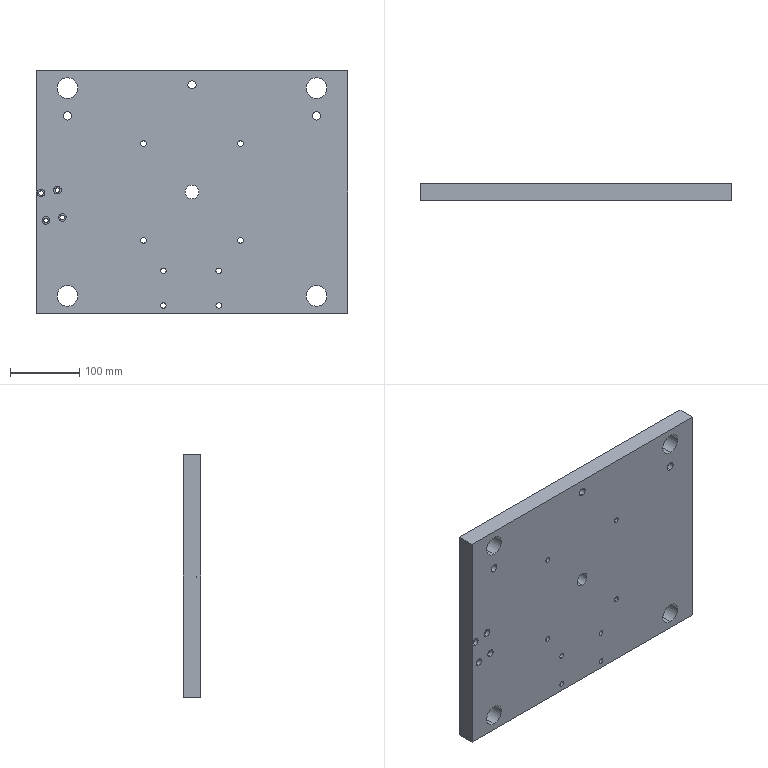Part | STEP file | OP10-102_base plate lower (L) | 1 solid | 74 faces | box 450 x 25 x 350 mm | volume 3834229 mm3 | cylinder 56 | plane 10 | cone 8 | commonest cylinder face diameters 8 x16 5 x8 6.6 x8 11 x8 30 x8 12 x6